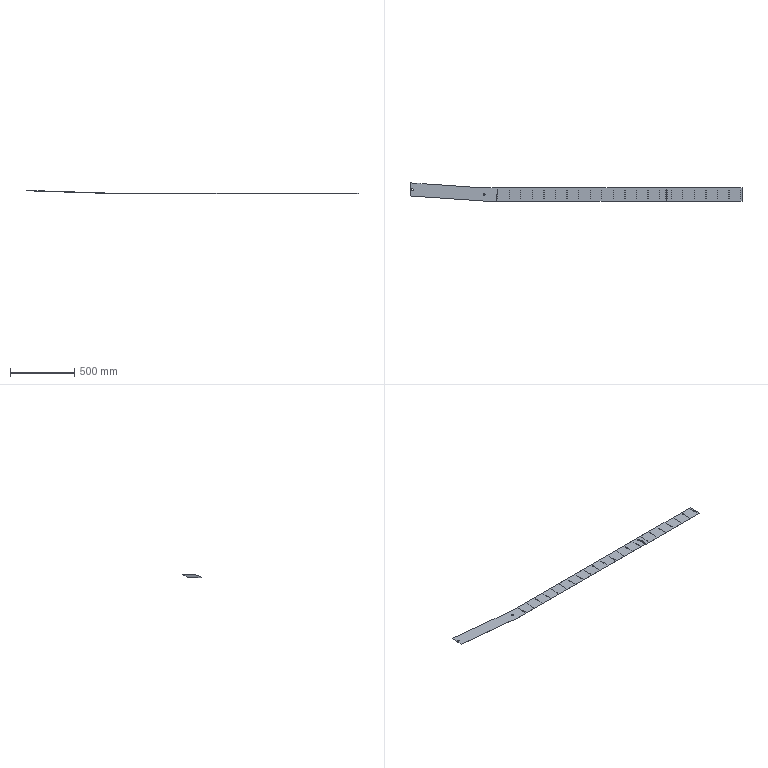Part | SolidWorks | features BaseBody 2 | 2 solids | 266 faces | box 2582 x 141.691 x 24.728 mm | volume 209802 mm3 | cylinder 246 | plane 18 | spline 2 | commonest cylinder face diameters 2.4 x240 15.3 x4 2 x1 3.6 x1